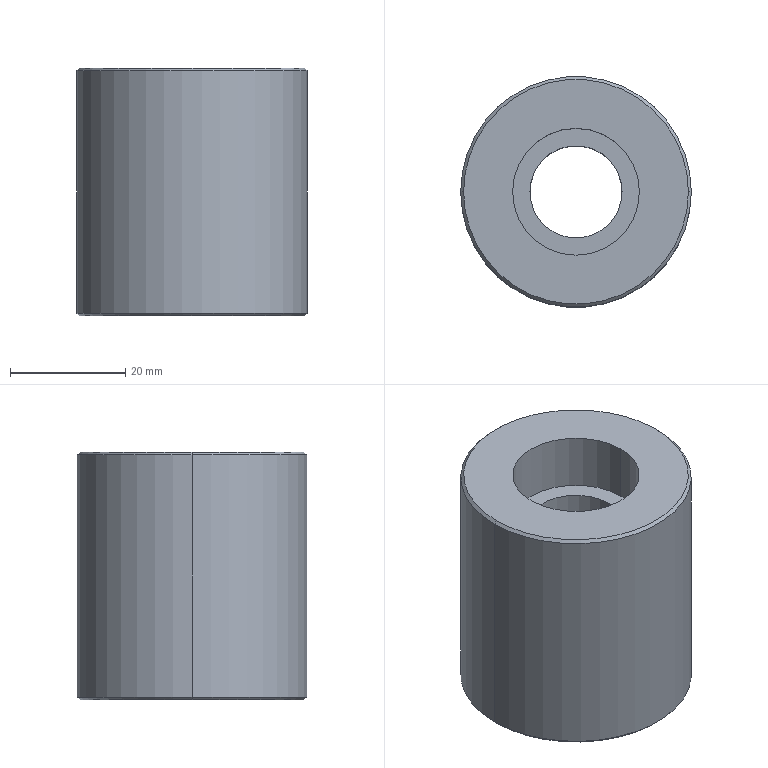Part | SolidWorks | features ICE 3, Chamfer 1, Extrusion 1 | 1 solid | 16 faces | box 40 x 40 x 43 mm | volume 42314 mm3 | cylinder 8 | cone 4 | plane 4 | commonest cylinder face diameters 22 x4 16 x2 40 x2
STEP:
#1=CARTESIAN_POINT('',(19.5,0.,43.));
#2=VERTEX_POINT('',#1);
#3=CARTESIAN_POINT('',(-19.5,0.,43.));
#4=VERTEX_POINT('',#3);
#5=CARTESIAN_POINT('',(0.,0.,43.));
#6=DIRECTION('',(0.,0.,1.));
#7=DIRECTION('',(1.,0.,0.));
#8=AXIS2_PLACEMENT_3D('',#5,#6,#7);
#9=CIRCLE('',#8,19.5);
#10=EDGE_CURVE('',#2,#4,#9,.T.);
#11=ORIENTED_EDGE('',*,*,#10,.F.);
#12=CARTESIAN_POINT('',(20.,0.,42.5));
#13=VERTEX_POINT('',#12);
#14=CARTESIAN_POINT('',(19.5,0.,43.));
#15=DIRECTION('',(0.7071,0.,-0.7071));
#16=VECTOR('',#15,1000.);
#17=LINE('',#14,#16);
#18=EDGE_CURVE('',#2,#13,#17,.T.);
#19=ORIENTED_EDGE('',*,*,#18,.T.);
#20=CARTESIAN_POINT('',(-20.,0.,42.5));
#21=VERTEX_POINT('',#20);
#22=CARTESIAN_POINT('',(0.,0.,42.5));
#23=DIRECTION('',(0.,0.,-1.));
#24=DIRECTION('',(1.,0.,0.));
#25=AXIS2_PLACEMENT_3D('',#22,#23,#24);
#26=CIRCLE('',#25,20.);
#27=EDGE_CURVE('',#21,#13,#26,.T.);
#28=ORIENTED_EDGE('',*,*,#27,.F.);
#29=CARTESIAN_POINT('',(-19.5,0.,43.));
#30=DIRECTION('',(-0.7071,0.,-0.7071));
#31=VECTOR('',#30,1000.);
#32=LINE('',#29,#31);
#33=EDGE_CURVE('',#4,#21,#32,.T.);
#34=ORIENTED_EDGE('',*,*,#33,.F.);
#35=EDGE_LOOP('',(#11,#19,#28,#34));
#36=FACE_OUTER_BOUND('',#35,.T.);
#37=CARTESIAN_POINT('',(0.,0.,43.));
#38=DIRECTION('',(0.,0.,-1.));
#39=DIRECTION('',(-1.,0.,0.));
#40=AXIS2_PLACEMENT_3D('',#37,#38,#39);
#41=CONICAL_SURFACE('',#40,19.5,0.7854);
#42=ADVANCED_FACE('',(#36),#41,.T.);
#43=CARTESIAN_POINT('',(-19.5,0.,0.));
#44=VERTEX_POINT('',#43);
#45=CARTESIAN_POINT('',(19.5,0.,0.));
#46=VERTEX_POINT('',#45);
#47=CARTESIAN_POINT('',(0.,0.,0.));
#48=DIRECTION('',(0.,0.,-1.));
#49=DIRECTION('',(1.,0.,0.));
#50=AXIS2_PLACEMENT_3D('',#47,#48,#49);
#51=CIRCLE('',#50,19.5);
#52=EDGE_CURVE('',#44,#46,#51,.T.);
#53=ORIENTED_EDGE('',*,*,#52,.F.);
#54=CARTESIAN_POINT('',(-20.,0.,0.5));
#55=VERTEX_POINT('',#54);
#56=CARTESIAN_POINT('',(-20.,0.,0.5));
#57=DIRECTION('',(-0.7071,0.,0.7071));
#58=VECTOR('',#57,1000.);
#59=LINE('',#56,#58);
#60=EDGE_CURVE('',#44,#55,#59,.T.);
#61=ORIENTED_EDGE('',*,*,#60,.T.);
#62=CARTESIAN_POINT('',(20.,0.,0.5));
#63=VERTEX_POINT('',#62);
#64=CARTESIAN_POINT('',(0.,0.,0.5));
#65=DIRECTION('',(0.,0.,1.));
#66=DIRECTION('',(1.,0.,0.));
#67=AXIS2_PLACEMENT_3D('',#64,#65,#66);
#68=CIRCLE('',#67,20.);
#69=EDGE_CURVE('',#63,#55,#68,.T.);
#70=ORIENTED_EDGE('',*,*,#69,.F.);
#71=CARTESIAN_POINT('',(20.,0.,0.5));
#72=DIRECTION('',(0.7071,0.,0.7071));
#73=VECTOR('',#72,1000.);
#74=LINE('',#71,#73);
#75=EDGE_CURVE('',#46,#63,#74,.T.);
#76=ORIENTED_EDGE('',*,*,#75,.F.);
#77=EDGE_LOOP('',(#53,#61,#70,#76));
#78=FACE_OUTER_BOUND('',#77,.T.);
#79=CARTESIAN_POINT('',(0.,0.,0.5));
#80=DIRECTION('',(0.,0.,1.));
#81=DIRECTION('',(1.,0.,0.));
#82=AXIS2_PLACEMENT_3D('',#79,#80,#81);
#83=CONICAL_SURFACE('',#82,20.,0.7854);
#84=ADVANCED_FACE('',(#78),#83,.T.);
#85=CARTESIAN_POINT('',(-8.,0.,33.));
#86=VERTEX_POINT('',#85);
#87=CARTESIAN_POINT('',(8.,0.,33.));
#88=VERTEX_POINT('',#87);
#89=CARTESIAN_POINT('',(0.,0.,33.));
#90=DIRECTION('',(0.,0.,1.));
#91=DIRECTION('',(1.,0.,0.));
#92=AXIS2_PLACEMENT_3D('',#89,#90,#91);
#93=CIRCLE('',#92,8.);
#94=EDGE_CURVE('',#86,#88,#93,.T.);
#95=ORIENTED_EDGE('',*,*,#94,.T.);
#96=CARTESIAN_POINT('',(8.,0.,7.));
#97=VERTEX_POINT('',#96);
#98=CARTESIAN_POINT('',(8.,0.,43.));
#99=DIRECTION('',(0.,0.,-1.));
#100=VECTOR('',#99,1000.);
#101=LINE('',#98,#100);
#102=EDGE_CURVE('',#88,#97,#101,.T.);
#103=ORIENTED_EDGE('',*,*,#102,.T.);
#104=CARTESIAN_POINT('',(-8.,0.,7.));
#105=VERTEX_POINT('',#104);
#106=CARTESIAN_POINT('',(0.,0.,7.));
#107=DIRECTION('',(0.,0.,-1.));
#108=DIRECTION('',(-1.,0.,0.));
#109=AXIS2_PLACEMENT_3D('',#106,#107,#108);
#110=CIRCLE('',#109,8.);
#111=EDGE_CURVE('',#97,#105,#110,.T.);
#112=ORIENTED_EDGE('',*,*,#111,.T.);
#113=CARTESIAN_POINT('',(-8.,0.,43.));
#114=DIRECTION('',(0.,0.,-1.));
#115=VECTOR('',#114,1000.);
#116=LINE('',#113,#115);
#117=EDGE_CURVE('',#86,#105,#116,.T.);
#118=ORIENTED_EDGE('',*,*,#117,.F.);
#119=EDGE_LOOP('',(#95,#103,#112,#118));
#120=FACE_OUTER_BOUND('',#119,.T.);
#121=CARTESIAN_POINT('',(0.,0.,43.));
#122=DIRECTION('',(0.,0.,-1.));
#123=DIRECTION('',(-1.,0.,0.));
#124=AXIS2_PLACEMENT_3D('',#121,#122,#123);
#125=CYLINDRICAL_SURFACE('',#124,8.);
#126=ADVANCED_FACE('',(#120),#125,.F.);
#127=CARTESIAN_POINT('',(11.,0.,7.));
#128=VERTEX_POINT('',#127);
#129=CARTESIAN_POINT('',(-11.,0.,7.));
#130=VERTEX_POINT('',#129);
#131=CARTESIAN_POINT('',(0.,0.,7.));
#132=DIRECTION('',(0.,0.,-1.));
#133=DIRECTION('',(-1.,0.,0.));
#134=AXIS2_PLACEMENT_3D('',#131,#132,#133);
#135=CIRCLE('',#134,11.);
#136=EDGE_CURVE('',#128,#130,#135,.T.);
#137=ORIENTED_EDGE('',*,*,#136,.F.);
#138=CARTESIAN_POINT('',(11.,0.,0.));
#139=VERTEX_POINT('',#138);
#140=CARTESIAN_POINT('',(11.,0.,7.));
#141=DIRECTION('',(0.,0.,-1.));
#142=VECTOR('',#141,1000.);
#143=LINE('',#140,#142);
#144=EDGE_CURVE('',#128,#139,#143,.T.);
#145=ORIENTED_EDGE('',*,*,#144,.T.);
#146=CARTESIAN_POINT('',(-11.,0.,0.));
#147=VERTEX_POINT('',#146);
#148=CARTESIAN_POINT('',(0.,0.,0.));
#149=DIRECTION('',(0.,0.,-1.));
#150=DIRECTION('',(-1.,0.,0.));
#151=AXIS2_PLACEMENT_3D('',#148,#149,#150);
#152=CIRCLE('',#151,11.);
#153=EDGE_CURVE('',#139,#147,#152,.T.);
#154=ORIENTED_EDGE('',*,*,#153,.T.);
#155=CARTESIAN_POINT('',(-11.,0.,7.));
#156=DIRECTION('',(0.,0.,-1.));
#157=VECTOR('',#156,1000.);
#158=LINE('',#155,#157);
#159=EDGE_CURVE('',#130,#147,#158,.T.);
#160=ORIENTED_EDGE('',*,*,#159,.F.);
#161=EDGE_LOOP('',(#137,#145,#154,#160));
#162=FACE_OUTER_BOUND('',#161,.T.);
#163=CARTESIAN_POINT('',(0.,0.,7.));
#164=DIRECTION('',(0.,0.,-1.));
#165=DIRECTION('',(-1.,0.,0.));
#166=AXIS2_PLACEMENT_3D('',#163,#164,#165);
#167=CYLINDRICAL_SURFACE('',#166,11.);
#168=ADVANCED_FACE('',(#162),#167,.F.);
#169=CARTESIAN_POINT('',(-11.,0.,33.));
#170=VERTEX_POINT('',#169);
#171=CARTESIAN_POINT('',(11.,0.,33.));
#172=VERTEX_POINT('',#171);
#173=CARTESIAN_POINT('',(0.,0.,33.));
#174=DIRECTION('',(0.,0.,1.));
#175=DIRECTION('',(1.,0.,0.));
#176=AXIS2_PLACEMENT_3D('',#173,#174,#175);
#177=CIRCLE('',#176,11.);
#178=EDGE_CURVE('',#170,#172,#177,.T.);
#179=ORIENTED_EDGE('',*,*,#178,.F.);
#180=CARTESIAN_POINT('',(-11.,0.,43.));
#181=VERTEX_POINT('',#180);
#182=CARTESIAN_POINT('',(-11.,0.,33.));
#183=DIRECTION('',(0.,0.,1.));
#184=VECTOR('',#183,1000.);
#185=LINE('',#182,#184);
#186=EDGE_CURVE('',#170,#181,#185,.T.);
#187=ORIENTED_EDGE('',*,*,#186,.T.);
#188=CARTESIAN_POINT('',(11.,0.,43.));
#189=VERTEX_POINT('',#188);
#190=CARTESIAN_POINT('',(0.,0.,43.));
#191=DIRECTION('',(0.,0.,1.));
#192=DIRECTION('',(1.,0.,0.));
#193=AXIS2_PLACEMENT_3D('',#190,#191,#192);
#194=CIRCLE('',#193,11.);
#195=EDGE_CURVE('',#181,#189,#194,.T.);
#196=ORIENTED_EDGE('',*,*,#195,.T.);
#197=CARTESIAN_POINT('',(11.,0.,33.));
#198=DIRECTION('',(0.,0.,1.));
#199=VECTOR('',#198,1000.);
#200=LINE('',#197,#199);
#201=EDGE_CURVE('',#172,#189,#200,.T.);
#202=ORIENTED_EDGE('',*,*,#201,.F.);
#203=EDGE_LOOP('',(#179,#187,#196,#202));
#204=FACE_OUTER_BOUND('',#203,.T.);
#205=CARTESIAN_POINT('',(0.,0.,33.));
#206=DIRECTION('',(0.,0.,1.));
#207=DIRECTION('',(1.,0.,0.));
#208=AXIS2_PLACEMENT_3D('',#205,#206,#207);
#209=CYLINDRICAL_SURFACE('',#208,11.);
#210=ADVANCED_FACE('',(#204),#209,.F.);
#211=ORIENTED_EDGE('',*,*,#27,.T.);
#212=CARTESIAN_POINT('',(20.,0.,43.));
#213=DIRECTION('',(0.,0.,-1.));
#214=VECTOR('',#213,1000.);
#215=LINE('',#212,#214);
#216=EDGE_CURVE('',#13,#63,#215,.T.);
#217=ORIENTED_EDGE('',*,*,#216,.T.);
#218=ORIENTED_EDGE('',*,*,#69,.T.);
#219=CARTESIAN_POINT('',(-20.,0.,43.));
#220=DIRECTION('',(0.,0.,-1.));
#221=VECTOR('',#220,1000.);
#222=LINE('',#219,#221);
#223=EDGE_CURVE('',#21,#55,#222,.T.);
#224=ORIENTED_EDGE('',*,*,#223,.F.);
#225=EDGE_LOOP('',(#211,#217,#218,#224));
#226=FACE_OUTER_BOUND('',#225,.T.);
#227=CARTESIAN_POINT('',(0.,0.,43.));
#228=DIRECTION('',(0.,0.,-1.));
#229=DIRECTION('',(-1.,0.,0.));
#230=AXIS2_PLACEMENT_3D('',#227,#228,#229);
#231=CYLINDRICAL_SURFACE('',#230,20.);
#232=ADVANCED_FACE('',(#226),#231,.T.);
#233=ORIENTED_EDGE('',*,*,#216,.F.);
#234=CARTESIAN_POINT('',(0.,0.,42.5));
#235=DIRECTION('',(0.,0.,-1.));
#236=DIRECTION('',(1.,0.,0.));
#237=AXIS2_PLACEMENT_3D('',#234,#235,#236);
#238=CIRCLE('',#237,20.);
#239=EDGE_CURVE('',#13,#21,#238,.T.);
#240=ORIENTED_EDGE('',*,*,#239,.T.);
#241=ORIENTED_EDGE('',*,*,#223,.T.);
#242=CARTESIAN_POINT('',(0.,0.,0.5));
#243=DIRECTION('',(0.,0.,1.));
#244=DIRECTION('',(1.,0.,0.));
#245=AXIS2_PLACEMENT_3D('',#242,#243,#244);
#246=CIRCLE('',#245,20.);
#247=EDGE_CURVE('',#55,#63,#246,.T.);
#248=ORIENTED_EDGE('',*,*,#247,.T.);
#249=EDGE_LOOP('',(#233,#240,#241,#248));
#250=FACE_OUTER_BOUND('',#249,.T.);
#251=CARTESIAN_POINT('',(0.,0.,43.));
#252=DIRECTION('',(0.,0.,-1.));
#253=DIRECTION('',(-1.,0.,0.));
#254=AXIS2_PLACEMENT_3D('',#251,#252,#253);
#255=CYLINDRICAL_SURFACE('',#254,20.);
#256=ADVANCED_FACE('',(#250),#255,.T.);
#257=CARTESIAN_POINT('',(0.,0.,43.));
#258=DIRECTION('',(0.,0.,1.));
#259=DIRECTION('',(1.,0.,0.));
#260=AXIS2_PLACEMENT_3D('',#257,#258,#259);
#261=CIRCLE('',#260,19.5);
#262=EDGE_CURVE('',#4,#2,#261,.T.);
#263=ORIENTED_EDGE('',*,*,#262,.T.);
#264=ORIENTED_EDGE('',*,*,#10,.T.);
#265=EDGE_LOOP('',(#263,#264));
#266=FACE_OUTER_BOUND('',#265,.T.);
#267=CARTESIAN_POINT('',(0.,0.,43.));
#268=DIRECTION('',(0.,0.,1.));
#269=DIRECTION('',(1.,0.,0.));
#270=AXIS2_PLACEMENT_3D('',#267,#268,#269);
#271=CIRCLE('',#270,11.);
#272=EDGE_CURVE('',#189,#181,#271,.T.);
#273=ORIENTED_EDGE('',*,*,#272,.F.);
#274=ORIENTED_EDGE('',*,*,#195,.F.);
#275=EDGE_LOOP('',(#273,#274));
#276=FACE_BOUND('',#275,.T.);
#277=CARTESIAN_POINT('',(0.,0.,43.));
#278=DIRECTION('',(0.,0.,1.));
#279=DIRECTION('',(1.,0.,0.));
#280=AXIS2_PLACEMENT_3D('',#277,#278,#279);
#281=PLANE('',#280);
#282=ADVANCED_FACE('',(#266,#276),#281,.T.);
#283=CARTESIAN_POINT('',(0.,0.,0.));
#284=DIRECTION('',(0.,0.,-1.));
#285=DIRECTION('',(1.,0.,0.));
#286=AXIS2_PLACEMENT_3D('',#283,#284,#285);
#287=CIRCLE('',#286,19.5);
#288=EDGE_CURVE('',#46,#44,#287,.T.);
#289=ORIENTED_EDGE('',*,*,#288,.T.);
#290=ORIENTED_EDGE('',*,*,#52,.T.);
#291=EDGE_LOOP('',(#289,#290));
#292=FACE_OUTER_BOUND('',#291,.T.);
#293=CARTESIAN_POINT('',(0.,0.,0.));
#294=DIRECTION('',(0.,0.,-1.));
#295=DIRECTION('',(-1.,0.,0.));
#296=AXIS2_PLACEMENT_3D('',#293,#294,#295);
#297=CIRCLE('',#296,11.);
#298=EDGE_CURVE('',#147,#139,#297,.T.);
#299=ORIENTED_EDGE('',*,*,#298,.F.);
#300=ORIENTED_EDGE('',*,*,#153,.F.);
#301=EDGE_LOOP('',(#299,#300));
#302=FACE_BOUND('',#301,.T.);
#303=CARTESIAN_POINT('',(0.,0.,0.));
#304=DIRECTION('',(0.,0.,1.));
#305=DIRECTION('',(1.,0.,0.));
#306=AXIS2_PLACEMENT_3D('',#303,#304,#305);
#307=PLANE('',#306);
#308=ADVANCED_FACE('',(#292,#302),#307,.F.);
#309=ORIENTED_EDGE('',*,*,#186,.F.);
#310=CARTESIAN_POINT('',(0.,0.,33.));
#311=DIRECTION('',(0.,0.,1.));
#312=DIRECTION('',(1.,0.,0.));
#313=AXIS2_PLACEMENT_3D('',#310,#311,#312);
#314=CIRCLE('',#313,11.);
#315=EDGE_CURVE('',#172,#170,#314,.T.);
#316=ORIENTED_EDGE('',*,*,#315,.F.);
#317=ORIENTED_EDGE('',*,*,#201,.T.);
#318=ORIENTED_EDGE('',*,*,#272,.T.);
#319=EDGE_LOOP('',(#309,#316,#317,#318));
#320=FACE_OUTER_BOUND('',#319,.T.);
#321=CARTESIAN_POINT('',(0.,0.,33.));
#322=DIRECTION('',(0.,0.,1.));
#323=DIRECTION('',(1.,0.,0.));
#324=AXIS2_PLACEMENT_3D('',#321,#322,#323);
#325=CYLINDRICAL_SURFACE('',#324,11.);
#326=ADVANCED_FACE('',(#320),#325,.F.);
#327=ORIENTED_EDGE('',*,*,#94,.F.);
#328=CARTESIAN_POINT('',(0.,0.,33.));
#329=DIRECTION('',(0.,0.,1.));
#330=DIRECTION('',(1.,0.,0.));
#331=AXIS2_PLACEMENT_3D('',#328,#329,#330);
#332=CIRCLE('',#331,8.);
#333=EDGE_CURVE('',#88,#86,#332,.T.);
#334=ORIENTED_EDGE('',*,*,#333,.F.);
#335=EDGE_LOOP('',(#327,#334));
#336=FACE_BOUND('',#335,.T.);
#337=ORIENTED_EDGE('',*,*,#315,.T.);
#338=ORIENTED_EDGE('',*,*,#178,.T.);
#339=EDGE_LOOP('',(#337,#338));
#340=FACE_OUTER_BOUND('',#339,.T.);
#341=CARTESIAN_POINT('',(0.,0.,33.));
#342=DIRECTION('',(0.,0.,1.));
#343=DIRECTION('',(1.,0.,0.));
#344=AXIS2_PLACEMENT_3D('',#341,#342,#343);
#345=PLANE('',#344);
#346=ADVANCED_FACE('',(#336,#340),#345,.T.);
#347=ORIENTED_EDGE('',*,*,#144,.F.);
#348=CARTESIAN_POINT('',(0.,0.,7.));
#349=DIRECTION('',(0.,0.,-1.));
#350=DIRECTION('',(-1.,0.,0.));
#351=AXIS2_PLACEMENT_3D('',#348,#349,#350);
#352=CIRCLE('',#351,11.);
#353=EDGE_CURVE('',#130,#128,#352,.T.);
#354=ORIENTED_EDGE('',*,*,#353,.F.);
#355=ORIENTED_EDGE('',*,*,#159,.T.);
#356=ORIENTED_EDGE('',*,*,#298,.T.);
#357=EDGE_LOOP('',(#347,#354,#355,#356));
#358=FACE_OUTER_BOUND('',#357,.T.);
#359=CARTESIAN_POINT('',(0.,0.,7.));
#360=DIRECTION('',(0.,0.,-1.));
#361=DIRECTION('',(-1.,0.,0.));
#362=AXIS2_PLACEMENT_3D('',#359,#360,#361);
#363=CYLINDRICAL_SURFACE('',#362,11.);
#364=ADVANCED_FACE('',(#358),#363,.F.);
#365=CARTESIAN_POINT('',(0.,0.,7.));
#366=DIRECTION('',(0.,0.,-1.));
#367=DIRECTION('',(-1.,0.,0.));
#368=AXIS2_PLACEMENT_3D('',#365,#366,#367);
#369=CIRCLE('',#368,8.);
#370=EDGE_CURVE('',#105,#97,#369,.T.);
#371=ORIENTED_EDGE('',*,*,#370,.F.);
#372=ORIENTED_EDGE('',*,*,#111,.F.);
#373=EDGE_LOOP('',(#371,#372));
#374=FACE_BOUND('',#373,.T.);
#375=ORIENTED_EDGE('',*,*,#353,.T.);
#376=ORIENTED_EDGE('',*,*,#136,.T.);
#377=EDGE_LOOP('',(#375,#376));
#378=FACE_OUTER_BOUND('',#377,.T.);
#379=CARTESIAN_POINT('',(0.,0.,7.));
#380=DIRECTION('',(0.,0.,-1.));
#381=DIRECTION('',(-1.,0.,0.));
#382=AXIS2_PLACEMENT_3D('',#379,#380,#381);
#383=PLANE('',#382);
#384=ADVANCED_FACE('',(#374,#378),#383,.T.);
#385=ORIENTED_EDGE('',*,*,#102,.F.);
#386=ORIENTED_EDGE('',*,*,#333,.T.);
#387=ORIENTED_EDGE('',*,*,#117,.T.);
#388=ORIENTED_EDGE('',*,*,#370,.T.);
#389=EDGE_LOOP('',(#385,#386,#387,#388));
#390=FACE_OUTER_BOUND('',#389,.T.);
#391=CARTESIAN_POINT('',(0.,0.,43.));
#392=DIRECTION('',(0.,0.,-1.));
#393=DIRECTION('',(-1.,0.,0.));
#394=AXIS2_PLACEMENT_3D('',#391,#392,#393);
#395=CYLINDRICAL_SURFACE('',#394,8.);
#396=ADVANCED_FACE('',(#390),#395,.F.);
#397=ORIENTED_EDGE('',*,*,#60,.F.);
#398=ORIENTED_EDGE('',*,*,#288,.F.);
#399=ORIENTED_EDGE('',*,*,#75,.T.);
#400=ORIENTED_EDGE('',*,*,#247,.F.);
#401=EDGE_LOOP('',(#397,#398,#399,#400));
#402=FACE_OUTER_BOUND('',#401,.T.);
#403=CARTESIAN_POINT('',(0.,0.,0.5));
#404=DIRECTION('',(0.,0.,1.));
#405=DIRECTION('',(1.,0.,0.));
#406=AXIS2_PLACEMENT_3D('',#403,#404,#405);
#407=CONICAL_SURFACE('',#406,20.,0.7854);
#408=ADVANCED_FACE('',(#402),#407,.T.);
#409=ORIENTED_EDGE('',*,*,#18,.F.);
#410=ORIENTED_EDGE('',*,*,#262,.F.);
#411=ORIENTED_EDGE('',*,*,#33,.T.);
#412=ORIENTED_EDGE('',*,*,#239,.F.);
#413=EDGE_LOOP('',(#409,#410,#411,#412));
#414=FACE_OUTER_BOUND('',#413,.T.);
#415=CARTESIAN_POINT('',(0.,0.,43.));
#416=DIRECTION('',(0.,0.,-1.));
#417=DIRECTION('',(-1.,0.,0.));
#418=AXIS2_PLACEMENT_3D('',#415,#416,#417);
#419=CONICAL_SURFACE('',#418,19.5,0.7854);
#420=ADVANCED_FACE('',(#414),#419,.T.);
#421=CLOSED_SHELL('',(#42,#84,#126,#168,#210,#232,#256,#282,#308,#326,#346,#364,#384,#396,#408,#420));
#422=MANIFOLD_SOLID_BREP('',#421);
#423=CARTESIAN_POINT('',(0.,0.,0.));
#424=DIRECTION('',(0.,0.,1.));
#425=DIRECTION('',(1.,0.,0.));
#426=AXIS2_PLACEMENT_3D('',#423,#424,#425);
#427=(LENGTH_UNIT()NAMED_UNIT(*)SI_UNIT(.MILLI.,.METRE.));
#428=UNCERTAINTY_MEASURE_WITH_UNIT(LENGTH_MEASURE(0.00001),#427,'','');
#429=(NAMED_UNIT(*)PLANE_ANGLE_UNIT()SI_UNIT($,.RADIAN.));
#430=(NAMED_UNIT(*)SI_UNIT($,.STERADIAN.)SOLID_ANGLE_UNIT());
#431=(GEOMETRIC_REPRESENTATION_CONTEXT(3)GLOBAL_UNCERTAINTY_ASSIGNED_CONTEXT((#428))GLOBAL_UNIT_ASSIGNED_CONTEXT((#427,#429,#430))REPRESENTATION_CONTEXT('',''));
#432=ADVANCED_BREP_SHAPE_REPRESENTATION('',(#422,#426),#431);